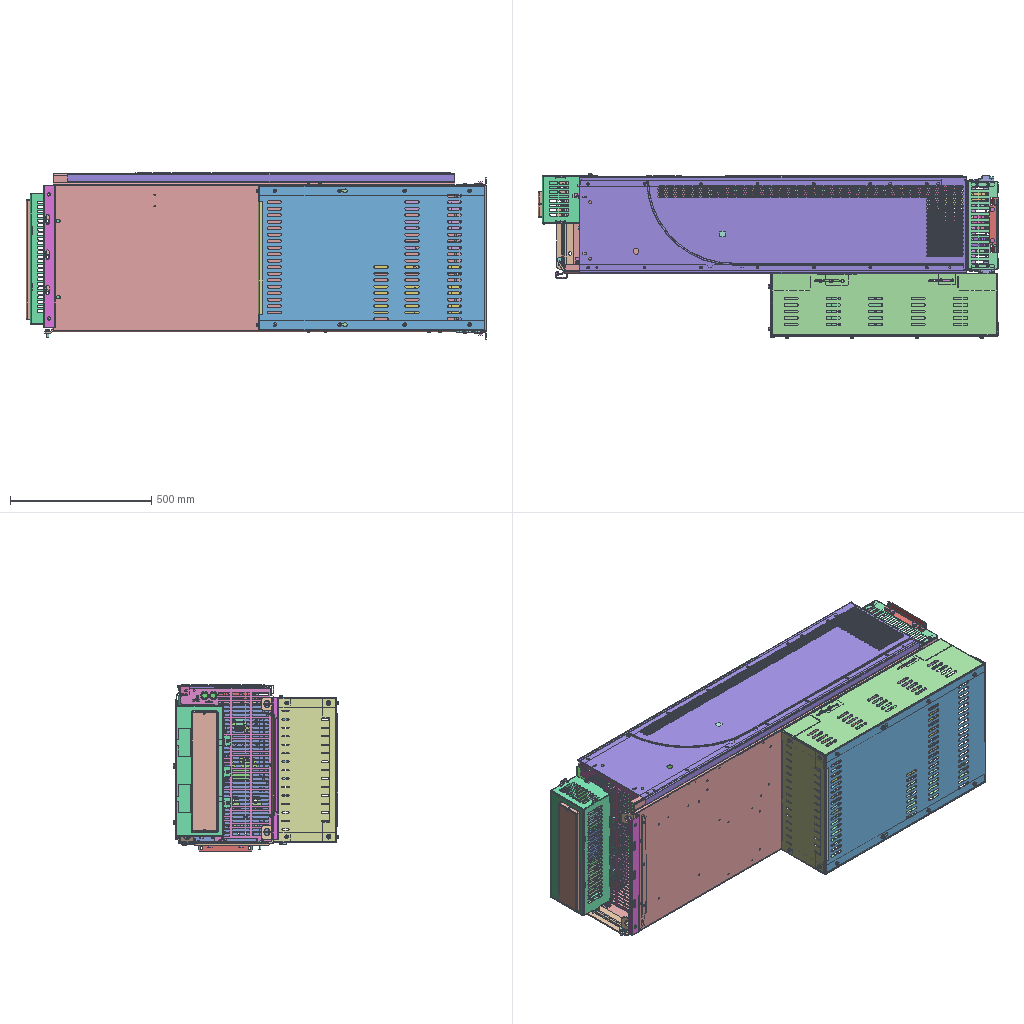Assembly | STEP file | 121 different items | 508 placed | box 1629 x 585 x 589 mm
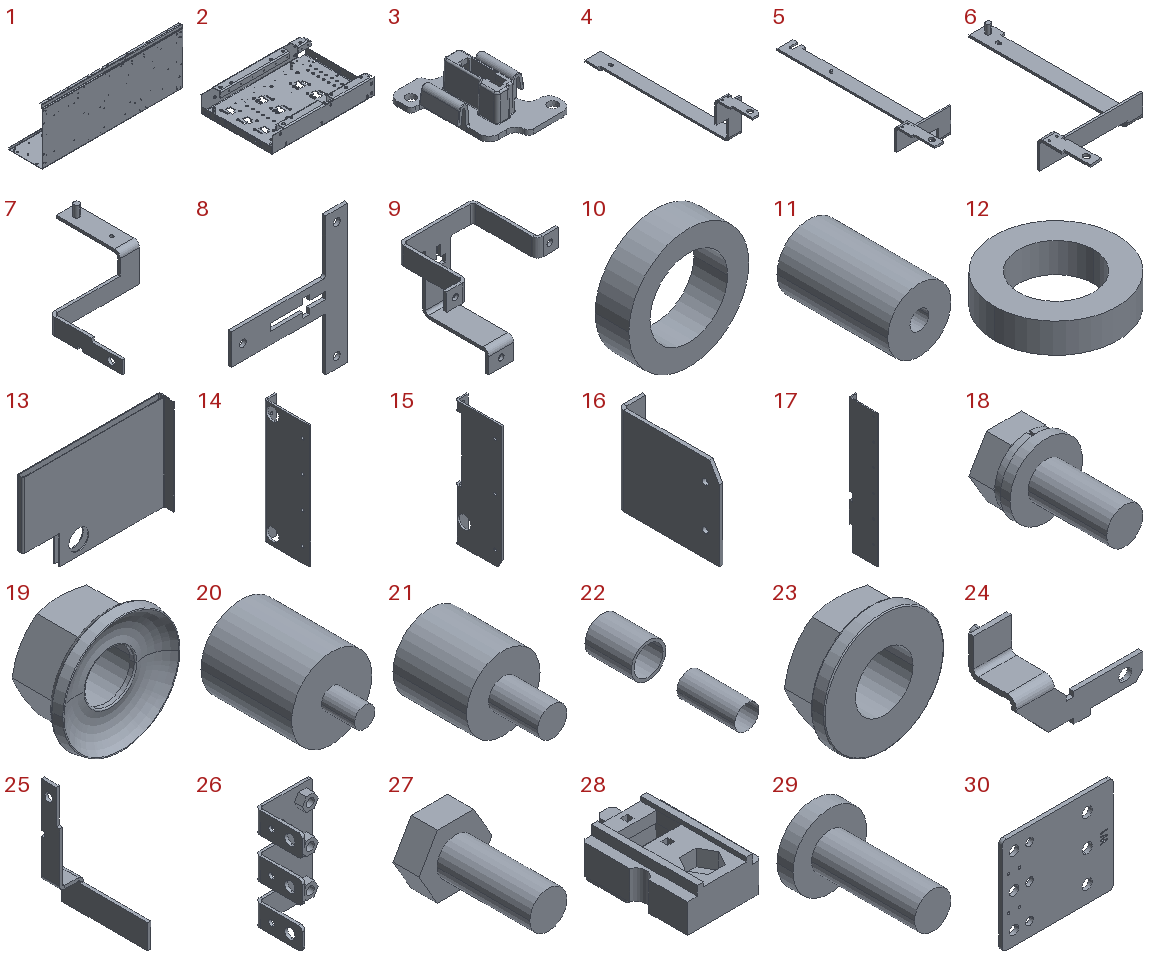Parts list (item | name | quantity | parent item | size | volume):
1 | 64741527 | x1 | - | 1421 x 347.5 x 560 mm | 3305754 mm3
2 | 64560280 | x1 | in 64640828_ASM | 493.5 x 340.5 x 93 mm | 732862 mm3
3 | 64534459 | x6 | in 64640828_ASM | 53 x 64.6 x 22 mm | 11629 mm3
4 | 64562487 | x1 | in 64640828_ASM | 67.1 x 477 x 136.5 mm | 104074 mm3
5 | 64562495 | x1 | in 64640828_ASM | 155.9 x 532.25 x 101.5 mm | 122513 mm3
6 | 64562509 | x1 | in 64640828_ASM | 233.8 x 450 x 76.5 mm | 121760 mm3
7 | 64560433 | x1 | in 64640828_ASM | 159.4 x 245 x 87.7 mm | 67125 mm3
8 | 64562894 | x1 | in 64564421_ASM | 132 x 4 x 157 mm | 27692 mm3
9 | 64562878 | x1 | in 64564421_ASM | 157 x 94 x 132 mm | 57021 mm3
10 | W468 | x1 | in 64564421_ASM | 108.1 x 30.3 x 108.1 mm | 161481 mm3
11 | LIB_58914274 | x3 | in 64564421_ASM | 20 x 35 x 20 mm | 10543 mm3
12 | FERRIITI_104 | x1 | in 64564421_ASM | 104 x 104 x 25 mm | 134441 mm3
13 | 64563181 | x1 | in 64640828_ASM | 151.5 x 16.5 x 101 mm | 21611 mm3
14 | 64605500 | x1 | in 64640828_ASM | 17.5 x 72.5 x 196.5 mm | 40557 mm3
15 | 64605526 | x1 | in 64640828_ASM | 17.5 x 72.5 x 194 mm | 34813 mm3
16 | 64605534 | x1 | in 64640828_ASM | 17.5 x 72.5 x 62.5 mm | 13245 mm3
17 | 64605551 | x1 | in 64640828_ASM | 17.5 x 72.5 x 328 mm | 65751 mm3
18 | LIB_36623110_M6X16 | x25 | in 64640828_ASM, 64667050_68233356_ASM, 68352100_LEFT_ASM, 68374154_ASM | 12 x 20 x 12 mm | 992.686 mm3
19 | KOPRESS_M10 | x5 | in 64640828_ASM | 20.951 x 11.146 x 20.951 mm | 1322 mm3
20 | LIB_57422564 | x1 | in 64640828_ASM | 19.5 x 30 x 19.5 mm | 6600 mm3
21 | SOLID | x2 | in LIB_64610121 | 15 x 25 x 15 mm | 2709 mm3
22 | COMPOUND | x2 | in LIB_64610121 | - | -
23 | LIB_68452317_M6_SERPRESS | x17 | in 64640828_ASM, 64634879_MITTAKUVA_ASM, 64564510_ASM, 64728113_MITTAKUVA_64801082_ASM | 12.5 x 5.2 x 12.5 mm | 351.327 mm3
24 | 64646443 | x1 | in 64640828_ASM | 133.75 x 65.3 x 88.252 mm | 33570 mm3
25 | 64646460 | x1 | in 64640828_ASM | 53.3 x 140.3 x 190 mm | 53459 mm3
26 | 64633074 | x3 | in 64639862_MITTAKUVA_64801082_AF2_ASM, 64639862_MITTAKUVA_64801082_AF1_ASM, 64639862_MITTAKUVA_64801082_AF0_ASM | 60.788 x 52 x 111.5 mm | 28803 mm3
27 | LIB_27897312_M10X25 | x9 | in 64639862_MITTAKUVA_64801082_AF2_ASM, 64639862_MITTAKUVA_64801082_AF1_ASM, 64639862_MITTAKUVA_64801082_AF0_ASM | 19.63 x 32 x 17 mm | 3715 mm3
28 | 58413461 | x9 | in 64639862_MITTAKUVA_64801082_AF2_ASM, 64639862_MITTAKUVA_64801082_AF1_ASM, 64639862_MITTAKUVA_64801082_AF0_ASM | 44 x 71 x 25 mm | 30731 mm3
29 | 4_8X13Y | x36 | in 64639862_MITTAKUVA_64801082_AF2_ASM, 64639862_MITTAKUVA_64801082_AF1_ASM, 64639862_MITTAKUVA_64801082_AF0_ASM | 9.3 x 16.348 x 9.3 mm | 389.106 mm3
30 | SOLID | x1 | in 64634861_AF2 | 144 x 5 x 125 mm | 84805 mm3
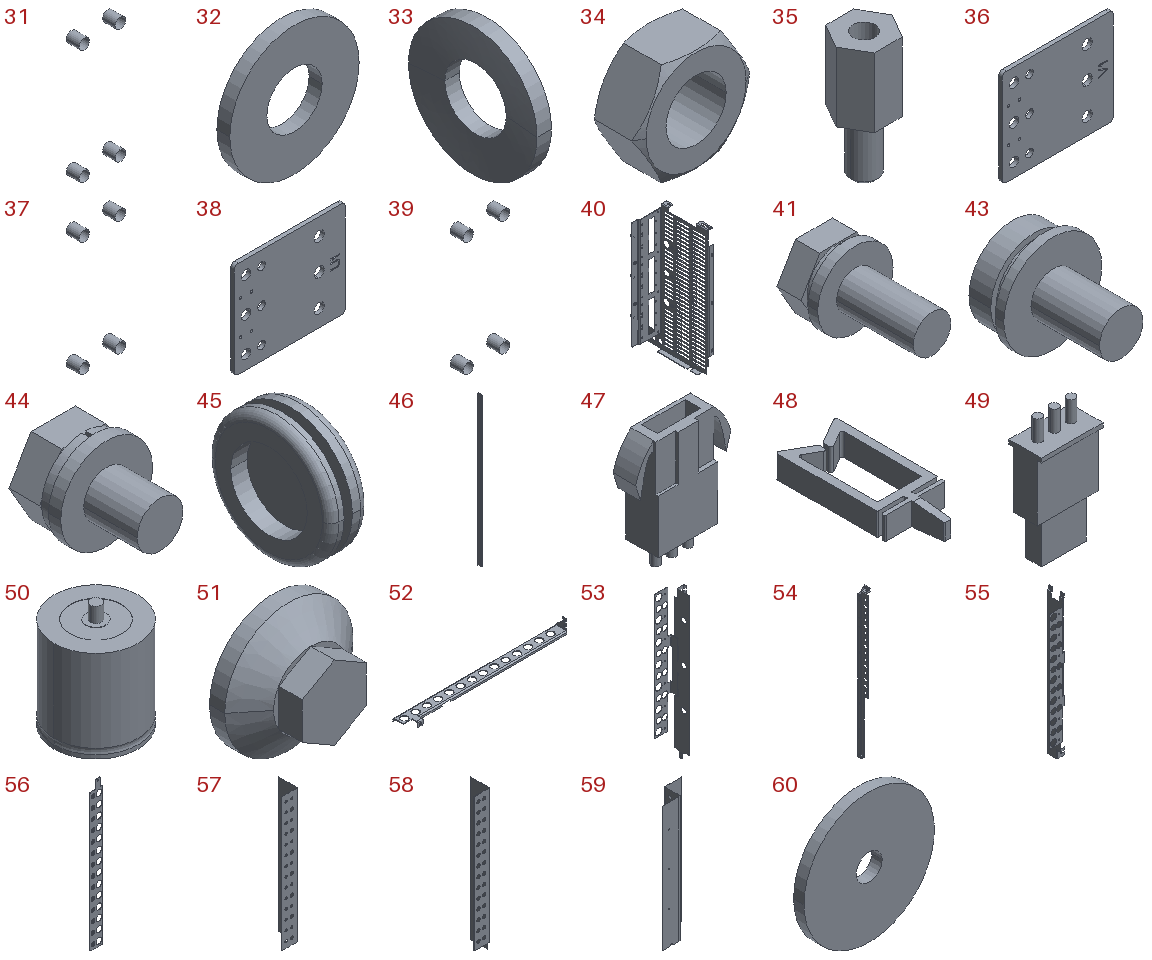31 | COMPOUND | x1 | in 64634861_AF2 | - | -
32 | M10_AALTOLAATTA_DIN125 | x9 | in 64639862_MITTAKUVA_64801082_AF2_ASM, 64639862_MITTAKUVA_64801082_AF1_ASM, 64639862_MITTAKUVA_64801082_AF0_ASM | 25 x 2.5 x 25 mm | 1002 mm3
33 | M10_PAINE_LAATTA | x9 | in 64639862_MITTAKUVA_64801082_AF2_ASM, 64639862_MITTAKUVA_64801082_AF1_ASM, 64639862_MITTAKUVA_64801082_AF0_ASM | 3.1 x 23 x 23 mm | 834.027 mm3
34 | LIB_27044239_HEX_NUT_M10_SIMPLE | x9 | in 64639862_MITTAKUVA_64801082_AF2_ASM, 64639862_MITTAKUVA_64801082_AF1_ASM, 64639862_MITTAKUVA_64801082_AF0_ASM | 19.63 x 8 x 17 mm | 1357 mm3
35 | 58411934 | x3 | in 64639862_MITTAKUVA_64801082_AF2_ASM, 64639862_MITTAKUVA_64801082_AF1_ASM, 64639862_MITTAKUVA_64801082_AF0_ASM | 8.091 x 7 x 18 mm | 467.745 mm3
36 | SOLID | x1 | in 64634861_AF1 | 144 x 5 x 125 mm | 84810 mm3
37 | COMPOUND | x1 | in 64634861_AF1 | - | -
38 | SOLID | x1 | in 64634861_AF0 | 144 x 5 x 125 mm | 84805 mm3
39 | COMPOUND | x1 | in 64634861_AF0 | - | -
40 | 64633091_AF0 | x1 | in 64634879_MITTAKUVA_ASM | 142 x 328 x 554.508 mm | 249746 mm3
41 | LIB_68310857_M10X25 | x25 | in 64634879_MITTAKUVA_ASM, 64667050_68233356_ASM, 64743368_MITTAKUVA_ASM | 20 x 31.4 x 20 mm | 4451 mm3
42 | 64637932_AF0 | x1 | in 64634879_MITTAKUVA_ASM | - | -
43 | LIB_68343097_M4X8 | x13 | in 64634879_MITTAKUVA_ASM | 9 x 11.088 x 9 mm | 282.702 mm3
44 | LIB_36623098_M6X10 | x24 | in 64634879_MITTAKUVA_ASM, 64564528_ASM, 64564536_ASM | 12 x 14 x 12 mm | 823.04 mm3
45 | 60008141 | x2 | in 64634879_MITTAKUVA_ASM | 9.25 x 30 x 30 mm | 3450 mm3
46 | 64685163 | x1 | in 64634879_MITTAKUVA_ASM | 4.361 x 13.946 x 520 mm | 14891 mm3
47 | ELR_03V | x1 | in 64634879_MITTAKUVA_ASM | 23.6 x 8.1 x 29.6 mm | 2454 mm3
48 | 10007151 | x4 | in 64634879_MITTAKUVA_ASM | 15 x 35.134 x 5.6 mm | 963.979 mm3
49 | ELP_03V | x1 | in 64634879_MITTAKUVA_ASM | 14.8 x 10.4 x 29.6 mm | 1903 mm3
50 | 90X105 | x14 | in 64564528_ASM, 64564536_ASM | 90 x 90 x 119.4 mm | 624644 mm3
51 | LIB_58129429 | x14 | in 64564528_ASM, 64564536_ASM | 38 x 19.45 x 38 mm | 10239 mm3
52 | 64560352 | x1 | in 64564528_ASM | 754 x 73 x 68.5 mm | 109655 mm3
53 | 64524275 | x1 | in 64564528_ASM | 128.478 x 101 x 779 mm | 142481 mm3
54 | 64560387 | x1 | in 64564536_ASM | 64 x 67 x 1316 mm | 321357 mm3
55 | 64524283 | x1 | in 64564536_ASM | 126.2 x 96.5 x 835.25 mm | 152034 mm3
56 | 64524267 | x1 | in 64564536_ASM | 64.7 x 6 x 771 mm | 38271 mm3
57 | 64524313 | x1 | in 64564536_ASM | 89 x 104.75 x 746 mm | 102676 mm3
58 | 68379539 | x1 | in 64564536_ASM | 86.7 x 104.75 x 786 mm | 103690 mm3
59 | 64524330 | x1 | in 64564510_ASM | 213.75 x 96 x 768 mm | 116112 mm3
60 | BAR_INSUL_25 | x3 | in 64564510_ASM | 25 x 2 x 25 mm | 942.478 mm3
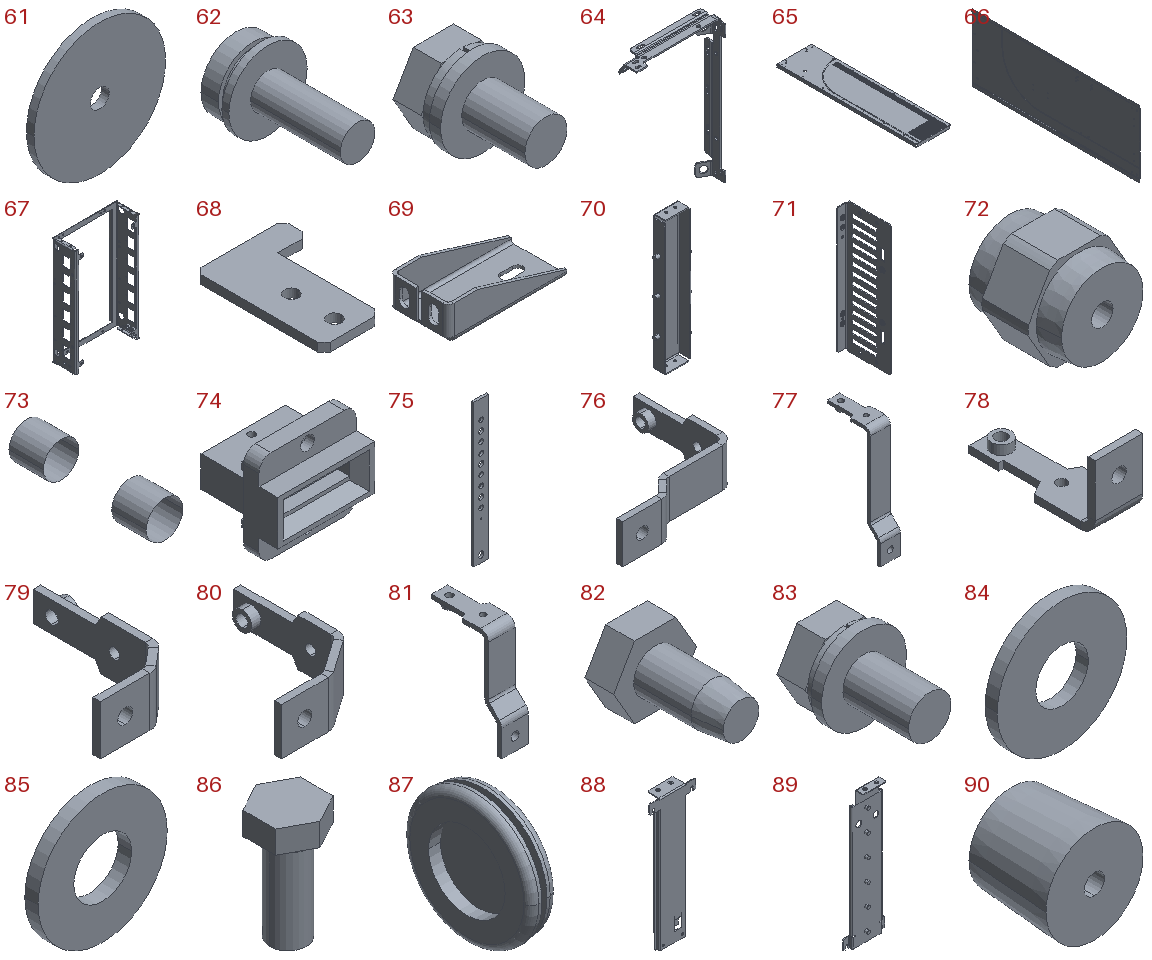61 | BAR_INSUL_35 | x3 | in 64564510_ASM | 35 x 2 x 35 mm | 1885 mm3
62 | LIB_68343071_M4X12 | x3 | in 64564510_ASM | 9 x 15.088 x 9 mm | 332.967 mm3
63 | LIB_36623101_M6X12 | x9 | in 64564510_ASM, 64667050_68233356_ASM, 68341477_ASM | 12 x 16 x 12 mm | 879.589 mm3
64 | 68352819 | x1 | - | 333 x 78.764 x 522.5 mm | 245441 mm3
65 | 64635212 | x1 | - | 342.5 x 1370 x 32 mm | 739959 mm3
66 | 64741551 | x1 | - | 17.8 x 1370 x 552 mm | 1150398 mm3
67 | 64604911 | x1 | in 64667050_68233356_ASM | 312 x 121 x 517 mm | 386207 mm3
68 | 64586793 | x2 | in 64667050_68233356_ASM | 40.84 x 60 x 4 mm | 6725 mm3
69 | 64644335 | x2 | in 64667050_68233356_ASM | 80.5 x 40 x 23.5 mm | 11043 mm3
70 | 64605046 | x1 | in 64667050_68233356_ASM | 80.6 x 27.5 x 306 mm | 73522 mm3
71 | 64586742 | x2 | in 64667050_68233356_ASM | 24 x 108 x 312 mm | 61627 mm3
72 | SOLID | x6 | in LIB_64575945 | 33 x 30 x 30 mm | 19613 mm3
73 | COMPOUND | x6 | in LIB_64575945 | - | -
74 | BUSHING_INSULATOR_CXBY | x12 | in 64667050_68233356_ASM | 56.5 x 48.5 x 53.5 mm | 51454 mm3
75 | 64586807 | x6 | in 64667050_68233356_ASM | 40 x 6 x 397.5 mm | 86530 mm3
76 | 64661426 | x1 | in 64667050_68233356_ASM | 130.6 x 113.5 x 40 mm | 49498 mm3
77 | 64586874 | x1 | in 64667050_68233356_ASM | 40 x 113.5 x 229 mm | 72622 mm3
78 | 64586840 | x1 | in 64667050_68233356_ASM | 40 x 113.5 x 55.6 mm | 32574 mm3
79 | 64586823 | x1 | in 64667050_68233356_ASM | 73.3 x 113.5 x 40 mm | 34639 mm3
80 | 64586815 | x1 | in 64667050_68233356_ASM | 79 x 113.5 x 40 mm | 36513 mm3
81 | 64586785 | x1 | in 64667050_68233356_ASM | 40 x 113.5 x 154 mm | 54622 mm3
82 | TAP_SCREW_DIN7500D_M6X12_TORX | x18 | in 64667050_68233356_ASM | 11.547 x 16 x 10 mm | 601.829 mm3
83 | LIB_36623152_M8X16 | x6 | in 64667050_68233356_ASM | 16 x 21.3 x 16 mm | 2046 mm3
84 | LIB_26379326_WASHER_M12 | x18 | in 64667050_68233356_ASM, 64743368_MITTAKUVA_ASM | 32 x 3 x 32 mm | 2015 mm3
85 | LIB_29542724_CUP_SPRING_M12 | x12 | in 64667050_68233356_ASM, 64743368_MITTAKUVA_ASM | 29 x 3 x 29 mm | 1583 mm3
86 | M12-30 | x6 | in 64667050_68233356_ASM | 19 x 21.1 x 38.1 mm | 5809 mm3
87 | 60008159 | x4 | in 64667050_68233356_ASM | 7.4 x 34.5 x 34.5 mm | 3903 mm3
88 | 64728407 | x1 | in 64728113_MITTAKUVA_64801082_ASM | 144 x 40 x 412 mm | 121719 mm3
89 | 64728377 | x1 | in 64728113_MITTAKUVA_64801082_ASM | 144 x 40.05 x 477.1 mm | 161672 mm3
90 | SOLID | x6 | in 09707255 | 41 x 35 x 41 mm | 39118 mm3
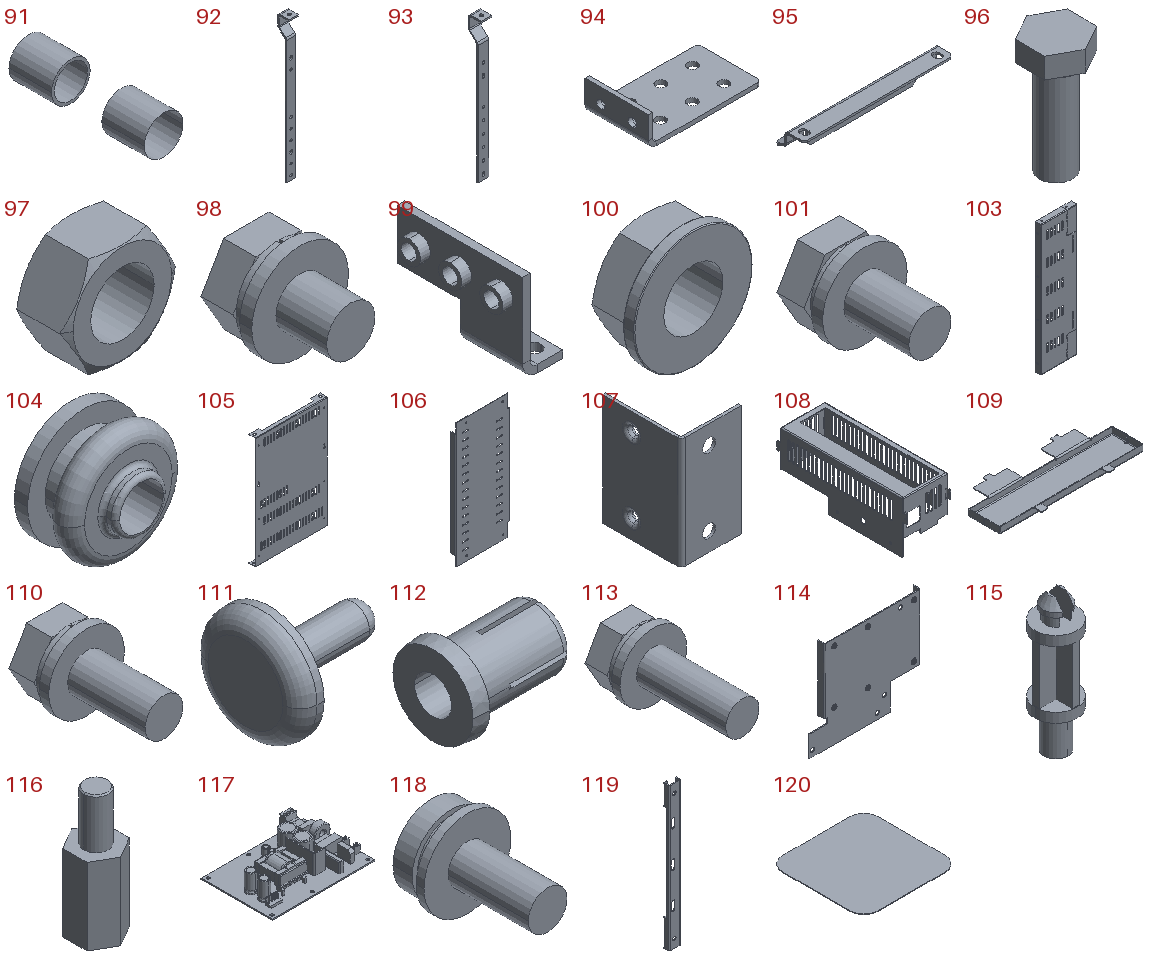91 | COMPOUND | x6 | in 09707255 | - | -
92 | 64805991 | x3 | in 64728113_MITTAKUVA_64801082_ASM | 40 x 51 x 631 mm | 163842 mm3
93 | 64806017 | x3 | in 64728113_MITTAKUVA_64801082_ASM | 40 x 51 x 542 mm | 142711 mm3
94 | 64728105 | x6 | in 64728113_MITTAKUVA_64801082_ASM | 160 x 90 x 44 mm | 97871 mm3
95 | 64668005 | x2 | in 64743368_MITTAKUVA_ASM | 193 x 38.839 x 30 mm | 23240 mm3
96 | M12-35 | x6 | in 64743368_MITTAKUVA_ASM | 19 x 21.1 x 43.1 mm | 6374 mm3
97 | LIB_27044255_HEX_NUT_M12_SIMPLE | x6 | in 64743368_MITTAKUVA_ASM | 21.939 x 10 x 19 mm | 1972 mm3
98 | LIB_36623144_M8X12 | x4 | in 64743368_MITTAKUVA_ASM | 16 x 17.3 x 16 mm | 1844 mm3
99 | 64665871 | x1 | in 64743368_MITTAKUVA_ASM | 39.9 x 100 x 72 mm | 40755 mm3
100 | LIB_68452121_M8_SERPRESS | x2 | in 64743368_MITTAKUVA_ASM | 16 x 6.9 x 16 mm | 740.456 mm3
101 | LIB_68343151_M10X20 | x4 | in 64743368_MITTAKUVA_ASM | 20 x 26.4 x 20 mm | 4058 mm3
102 | 64801082_BRAKE_BUSBAR_ASM | x1 | - | - | -
103 | 68352126 | x2 | in 68352126_ASM | 220 x 35 x 800 mm | 401401 mm3
104 | 233_07_060_230 | x16 | in 68352126_ASM | 13 x 8 x 13 mm | 572.53 mm3
105 | 68352118 | x1 | in 68352100_LEFT_ASM | 514 x 50 x 805 mm | 820655 mm3
106 | 68336503 | x1 | in 68352100_LEFT_ASM | 222.5 x 22 x 512 mm | 244893 mm3
107 | 68332991 | x2 | in 68352100_LEFT_ASM | 32.3 x 42.3 x 60 mm | 6427 mm3
108 | 68341469 | x1 | in 68341477_ASM | 195 x 489 x 195 mm | 358150 mm3
109 | 68341485 | x1 | in 68341477_ASM | 425 x 174 x 22 mm | 133591 mm3
110 | LIB_36623161_M8X20 | x2 | in 68341477_ASM | 16 x 25.3 x 16 mm | 2247 mm3
111 | SR_4060B_1 | x4 | in SRVO_4060_CLOSE_ASM | 8.9 x 8 x 8 mm | 92.138 mm3
112 | SR_4060B_2 | x4 | in SRVO_4060_CLOSE_ASM | 7 x 5.4 x 5.4 mm | 66.144 mm3
113 | LIB_36623179_M8X25 | x1 | - | 16 x 30.3 x 16 mm | 2498 mm3
114 | 68374120 | x1 | in 68374154_ASM | 189.45 x 13.5 x 155 mm | 38724 mm3
115 | MSCBSM_M4_8_01 | x5 | in 68374154_ASM | 7 x 7 x 22.9 mm | 355.891 mm3
116 | 49711204_74 | x1 | in 68374154_ASM | 7 x 8.09 x 20.9 mm | 569.977 mm3
117 | LIB_64668064 | x1 | in 68374154_ASM | 145 x 108.65 x 36.554 mm | 90051 mm3
118 | LIB_28112301_M4X10 | x1 | in 68374154_ASM | 9 x 13.088 x 9 mm | 307.834 mm3
119 | 68377927 | x1 | - | 41 x 21.5 x 500 mm | 101475 mm3
120 | 68423252 | x1 | - | 20 x 20 x 0.125 mm | 49.034 mm3
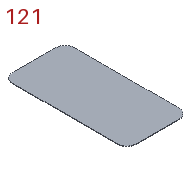121 | 68437831 | x1 | - | 20 x 40 x 0.125 mm | 99.034 mm3
Placements (level | parent | child | x y z in mm | rotation matrix by rows), first 274 of 546 lines:
1 | subassembly 2 | 64741527 | 0.0 0.0 0.0 | 1 0 0 0 1 0 0 0 1
1 | subassembly 2 | 64640828_ASM | 683.0 176.0 0.5 | 0 -1 0 1 0 0 0 0 1
2 | 64640828_ASM | 64560280 | -6.0 0.0 -1.0 | 0 1 0 0 0 -1 -1 0 0
2 | 64640828_ASM | 64534459 | 106.93 5.5 126.6 | 0 1 0 0 0 -1 -1 0 0
2 | 64640828_ASM | 64534459 | 26.23 5.5 126.6 | 0 1 0 0 0 -1 -1 0 0
2 | 64640828_ASM | 64534459 | -52.77 5.5 126.6 | 0 1 0 0 0 -1 -1 0 0
2 | 64640828_ASM | 64562487 | 91.18 29.5 -42.5 | 1 0 0 0 1 0 0 0 1
2 | 64640828_ASM | 64562495 | 50.78 35.5 -42.5 | 1 0 0 0 1 0 0 0 1
2 | 64640828_ASM | 64562509 | 11.83 41.5 -43.25 | 1 0 0 0 1 0 0 0 1
2 | 64640828_ASM | 64560433 | 39.33 60.5 -32.8 | 0 0 1 0 1 0 -1 0 0
2 | 64640828_ASM | 64564421_ASM | 108.8 41.5 -94.0 | 1 0 0 0 1 0 0 0 1
3 | 64564421_ASM | 64562894 | 0.0 0.0 0.0 | 1 0 0 0 1 0 0 0 1
3 | 64564421_ASM | 64562878 | -4.07 94.0 0.0 | 0 0 1 0 1 0 -1 0 0
3 | 64564421_ASM | W468 | -1.07 0.0 0.0 | 1 0 0 0 1 0 0 0 1
3 | 64564421_ASM | LIB_58914274 | 32.43 -39.0 66.0 | 1 0 0 0 1 0 0 0 1
3 | 64564421_ASM | LIB_58914274 | -74.57 -39.0 0.0 | 1 0 0 0 1 0 0 0 1
3 | 64564421_ASM | LIB_58914274 | 32.43 -39.0 -66.0 | 1 0 0 0 1 0 0 0 1
3 | 64564421_ASM | FERRIITI_104 | -1.07 90.0 0.0 | 1 0 0 0 0 -1 0 1 0
2 | 64640828_ASM | 64563181 | 123.83 30.5 -8.0 | 1 0 0 0 1 0 0 0 1
2 | 64640828_ASM | 64605500 | -139.0 -2.5 149.0 | 1 0 0 0 1 0 0 0 1
2 | 64640828_ASM | 64605526 | -139.0 -2.5 -89.5 | 1 0 0 0 1 0 0 0 1
2 | 64640828_ASM | 64605534 | 130.5 -2.5 -283.5 | -1 0 0 0 1 0 0 0 -1
2 | 64640828_ASM | 64605551 | 130.5 -2.5 -179.0 | -1 0 0 0 1 0 0 0 -1
2 | 64640828_ASM | LIB_36623110_M6X16 | 34.23 50.5 -94.0 | 1 0 0 0 1 0 0 0 1
2 | 64640828_ASM | LIB_36623110_M6X16 | 141.23 48.5 -160.0 | 1 0 0 0 1 0 0 0 1
2 | 64640828_ASM | LIB_36623110_M6X16 | 141.23 48.5 -28.0 | 1 0 0 0 1 0 0 0 1
2 | 64640828_ASM | KOPRESS_M10 | 84.93 157.5 -15.3 | 0 1 0 -1 0 0 0 0 1
2 | 64640828_ASM | KOPRESS_M10 | 107.23 392.0 -124.4 | 1 0 0 0 0 1 0 -1 0
2 | 64640828_ASM | KOPRESS_M10 | 114.03 365.0 -63.6 | -1 0 0 0 0 1 0 1 0
2 | 64640828_ASM | LIB_57422564 | 107.0 2.5 -73.5 | 1 0 0 0 1 0 0 0 1
2 | 64640828_ASM | LIB_64610121 | 107.23 335.5 -76.5 | 1 0 0 0 0 1 0 -1 0
3 | LIB_64610121 | SOLID | 0.0 0.0 0.0 | 1 0 0 0 1 0 0 0 1
3 | LIB_64610121 | COMPOUND | 0.0 0.0 0.0 | 1 0 0 0 1 0 0 0 1
2 | 64640828_ASM | LIB_64610121 | 107.23 362.5 -111.5 | -1 0 0 0 0 1 0 1 0
3 | LIB_64610121 | SOLID | 0.0 0.0 0.0 | 1 0 0 0 1 0 0 0 1
3 | LIB_64610121 | COMPOUND | 0.0 0.0 0.0 | 1 0 0 0 1 0 0 0 1
2 | 64640828_ASM | LIB_68452317_M6_SERPRESS | 107.23 335.5 -70.1 | -1 0 0 0 0 1 0 1 0
2 | 64640828_ASM | LIB_68452317_M6_SERPRESS | 107.23 362.5 -117.9 | 1 0 0 0 0 1 0 -1 0
2 | 64640828_ASM | 64534459 | -87.9 5.5 -5.0 | 0 -1 0 0 0 -1 1 0 0
2 | 64640828_ASM | 64534459 | -10.0 5.5 -5.0 | 0 -1 0 0 0 -1 1 0 0
2 | 64640828_ASM | 64534459 | 70.8 5.5 -5.0 | 0 -1 0 0 0 -1 1 0 0
2 | 64640828_ASM | 64646443 | 33.0 66.25 126.5 | 0 0 -1 -1 0 0 0 1 0
2 | 64640828_ASM | 64646460 | -70.0 -67.5 126.5 | 0 -1 0 0 0 -1 1 0 0
2 | 64640828_ASM | KOPRESS_M10 | 49.5 102.5 166.7 | -1 0 0 0 0 1 0 1 0
2 | 64640828_ASM | KOPRESS_M10 | 46.748 46.25 178.7 | -1 0 0 0 0 1 0 1 0
1 | subassembly 2 | 64634879_MITTAKUVA_ASM | -563.5 197.095 116.25 | 0 -1 0 -1 0 0 0 0 -1
2 | 64634879_MITTAKUVA_ASM | 64639862_MITTAKUVA_64801082_AF2_ASM | 0.0 0.0 0.0 | 1 0 0 0 1 0 0 0 1
3 | 64639862_MITTAKUVA_64801082_AF2_ASM | 64633074 | 0.0 0.0 0.0 | 1 0 0 0 1 0 0 0 1
3 | 64639862_MITTAKUVA_64801082_AF2_ASM | LIB_27897312_M10X25 | -37.065 -35.7 -44.5 | 0 1 0 1 0 0 0 0 -1
3 | 64639862_MITTAKUVA_64801082_AF2_ASM | LIB_27897312_M10X25 | -37.065 -35.7 0.0 | 0 1 0 1 0 0 0 0 -1
3 | 64639862_MITTAKUVA_64801082_AF2_ASM | LIB_27897312_M10X25 | -37.065 -35.7 44.5 | 0 1 0 1 0 0 0 0 -1
3 | 64639862_MITTAKUVA_64801082_AF2_ASM | 58413461 | -28.315 -18.0 -44.5 | 0 0 -1 0 1 0 1 0 0
3 | 64639862_MITTAKUVA_64801082_AF2_ASM | 58413461 | -28.315 -18.0 0.0 | 0 0 -1 0 1 0 1 0 0
3 | 64639862_MITTAKUVA_64801082_AF2_ASM | 58413461 | -28.315 -18.0 44.5 | 0 0 -1 0 1 0 1 0 0
3 | 64639862_MITTAKUVA_64801082_AF2_ASM | 4_8X13Y | -11.565 -42.0 -27.5 | 0 1 0 -1 0 0 0 0 1
3 | 64639862_MITTAKUVA_64801082_AF2_ASM | 4_8X13Y | -11.565 -42.0 17.0 | 0 1 0 -1 0 0 0 0 1
3 | 64639862_MITTAKUVA_64801082_AF2_ASM | 4_8X13Y | -11.565 -42.0 61.5 | 0 1 0 -1 0 0 0 0 1
3 | 64639862_MITTAKUVA_64801082_AF2_ASM | 4_8X13Y | -11.565 -42.0 -61.5 | 0 1 0 -1 0 0 0 0 1
3 | 64639862_MITTAKUVA_64801082_AF2_ASM | 4_8X13Y | -11.565 -42.0 -17.0 | 0 1 0 -1 0 0 0 0 1
3 | 64639862_MITTAKUVA_64801082_AF2_ASM | 4_8X13Y | -11.565 -42.0 27.5 | 0 1 0 -1 0 0 0 0 1
3 | 64639862_MITTAKUVA_64801082_AF2_ASM | 4_8X13Y | -11.565 17.5 -44.5 | 0 1 0 -1 0 0 0 0 1
3 | 64639862_MITTAKUVA_64801082_AF2_ASM | 4_8X13Y | -11.565 17.5 0.0 | 0 1 0 -1 0 0 0 0 1
3 | 64639862_MITTAKUVA_64801082_AF2_ASM | 4_8X13Y | -11.565 17.5 44.5 | 0 1 0 -1 0 0 0 0 1
3 | 64639862_MITTAKUVA_64801082_AF2_ASM | 4_8X13Y | -43.565 -15.5 -44.5 | 0 -1 0 1 0 0 0 0 1
3 | 64639862_MITTAKUVA_64801082_AF2_ASM | 4_8X13Y | -43.565 -15.5 0.0 | 0 -1 0 1 0 0 0 0 1
3 | 64639862_MITTAKUVA_64801082_AF2_ASM | 4_8X13Y | -43.565 -15.5 44.5 | 0 -1 0 1 0 0 0 0 1
3 | 64639862_MITTAKUVA_64801082_AF2_ASM | 64634861_AF2 | -45.065 21.3 0.0 | 0 1 0 1 0 0 0 0 -1
4 | 64634861_AF2 | SOLID | 0.0 0.0 0.0 | 1 0 0 0 1 0 0 0 1
4 | 64634861_AF2 | COMPOUND | 0.0 0.0 0.0 | 1 0 0 0 1 0 0 0 1
3 | 64639862_MITTAKUVA_64801082_AF2_ASM | M10_AALTOLAATTA_DIN125 | -47.565 -35.7 -44.5 | 0 1 0 -1 0 0 0 0 1
3 | 64639862_MITTAKUVA_64801082_AF2_ASM | M10_AALTOLAATTA_DIN125 | -47.565 -35.7 0.0 | 0 1 0 -1 0 0 0 0 1
3 | 64639862_MITTAKUVA_64801082_AF2_ASM | M10_AALTOLAATTA_DIN125 | -47.565 -35.7 44.5 | 0 1 0 -1 0 0 0 0 1
3 | 64639862_MITTAKUVA_64801082_AF2_ASM | M10_PAINE_LAATTA | -47.065 -35.7 -44.5 | -1 0 0 0 -1 0 0 0 1
3 | 64639862_MITTAKUVA_64801082_AF2_ASM | M10_PAINE_LAATTA | -47.065 -35.7 0.0 | -1 0 0 0 -1 0 0 0 1
3 | 64639862_MITTAKUVA_64801082_AF2_ASM | M10_PAINE_LAATTA | -47.065 -35.7 44.5 | -1 0 0 0 -1 0 0 0 1
3 | 64639862_MITTAKUVA_64801082_AF2_ASM | LIB_27044239_HEX_NUT_M10_SIMPLE | -58.065 -35.7 -44.5 | 0 1 0 -1 0 0 0 0 1
3 | 64639862_MITTAKUVA_64801082_AF2_ASM | LIB_27044239_HEX_NUT_M10_SIMPLE | -58.065 -35.7 0.0 | 0 1 0 -1 0 0 0 0 1
3 | 64639862_MITTAKUVA_64801082_AF2_ASM | LIB_27044239_HEX_NUT_M10_SIMPLE | -58.065 -35.7 44.5 | 0 1 0 -1 0 0 0 0 1
3 | 64639862_MITTAKUVA_64801082_AF2_ASM | 58411934 | -45.065 -28.7 -22.25 | 0 0 -1 -1 0 0 0 1 0
2 | 64634879_MITTAKUVA_ASM | 64639862_MITTAKUVA_64801082_AF1_ASM | 0.0 0.0 151.75 | 1 0 0 0 1 0 0 0 1
3 | 64639862_MITTAKUVA_64801082_AF1_ASM | 64633074 | 0.0 0.0 0.0 | 1 0 0 0 1 0 0 0 1
3 | 64639862_MITTAKUVA_64801082_AF1_ASM | LIB_27897312_M10X25 | -37.065 -35.7 -44.5 | 0 1 0 1 0 0 0 0 -1
3 | 64639862_MITTAKUVA_64801082_AF1_ASM | LIB_27897312_M10X25 | -37.065 -35.7 0.0 | 0 1 0 1 0 0 0 0 -1
3 | 64639862_MITTAKUVA_64801082_AF1_ASM | LIB_27897312_M10X25 | -37.065 -35.7 44.5 | 0 1 0 1 0 0 0 0 -1
3 | 64639862_MITTAKUVA_64801082_AF1_ASM | 58413461 | -28.315 -18.0 -44.5 | 0 0 -1 0 1 0 1 0 0
3 | 64639862_MITTAKUVA_64801082_AF1_ASM | 58413461 | -28.315 -18.0 0.0 | 0 0 -1 0 1 0 1 0 0
3 | 64639862_MITTAKUVA_64801082_AF1_ASM | 58413461 | -28.315 -18.0 44.5 | 0 0 -1 0 1 0 1 0 0
3 | 64639862_MITTAKUVA_64801082_AF1_ASM | 4_8X13Y | -11.565 -42.0 -27.5 | 0 1 0 -1 0 0 0 0 1
3 | 64639862_MITTAKUVA_64801082_AF1_ASM | 4_8X13Y | -11.565 -42.0 17.0 | 0 1 0 -1 0 0 0 0 1
3 | 64639862_MITTAKUVA_64801082_AF1_ASM | 4_8X13Y | -11.565 -42.0 61.5 | 0 1 0 -1 0 0 0 0 1
3 | 64639862_MITTAKUVA_64801082_AF1_ASM | 4_8X13Y | -11.565 -42.0 -61.5 | 0 1 0 -1 0 0 0 0 1
3 | 64639862_MITTAKUVA_64801082_AF1_ASM | 4_8X13Y | -11.565 -42.0 -17.0 | 0 1 0 -1 0 0 0 0 1
3 | 64639862_MITTAKUVA_64801082_AF1_ASM | 4_8X13Y | -11.565 -42.0 27.5 | 0 1 0 -1 0 0 0 0 1
3 | 64639862_MITTAKUVA_64801082_AF1_ASM | 4_8X13Y | -11.565 17.5 -44.5 | 0 1 0 -1 0 0 0 0 1
3 | 64639862_MITTAKUVA_64801082_AF1_ASM | 4_8X13Y | -11.565 17.5 0.0 | 0 1 0 -1 0 0 0 0 1
3 | 64639862_MITTAKUVA_64801082_AF1_ASM | 4_8X13Y | -11.565 17.5 44.5 | 0 1 0 -1 0 0 0 0 1
3 | 64639862_MITTAKUVA_64801082_AF1_ASM | 4_8X13Y | -43.565 -15.5 -44.5 | 0 -1 0 1 0 0 0 0 1
3 | 64639862_MITTAKUVA_64801082_AF1_ASM | 4_8X13Y | -43.565 -15.5 0.0 | 0 -1 0 1 0 0 0 0 1
3 | 64639862_MITTAKUVA_64801082_AF1_ASM | 4_8X13Y | -43.565 -15.5 44.5 | 0 -1 0 1 0 0 0 0 1
3 | 64639862_MITTAKUVA_64801082_AF1_ASM | 64634861_AF1 | -45.065 21.3 0.0 | 0 1 0 1 0 0 0 0 -1
4 | 64634861_AF1 | SOLID | 0.0 0.0 0.0 | 1 0 0 0 1 0 0 0 1
4 | 64634861_AF1 | COMPOUND | 0.0 0.0 0.0 | 1 0 0 0 1 0 0 0 1
3 | 64639862_MITTAKUVA_64801082_AF1_ASM | M10_AALTOLAATTA_DIN125 | -47.565 -35.7 -44.5 | 0 1 0 -1 0 0 0 0 1
3 | 64639862_MITTAKUVA_64801082_AF1_ASM | M10_AALTOLAATTA_DIN125 | -47.565 -35.7 0.0 | 0 1 0 -1 0 0 0 0 1
3 | 64639862_MITTAKUVA_64801082_AF1_ASM | M10_AALTOLAATTA_DIN125 | -47.565 -35.7 44.5 | 0 1 0 -1 0 0 0 0 1
3 | 64639862_MITTAKUVA_64801082_AF1_ASM | M10_PAINE_LAATTA | -47.065 -35.7 -44.5 | -1 0 0 0 -1 0 0 0 1
3 | 64639862_MITTAKUVA_64801082_AF1_ASM | M10_PAINE_LAATTA | -47.065 -35.7 0.0 | -1 0 0 0 -1 0 0 0 1
3 | 64639862_MITTAKUVA_64801082_AF1_ASM | M10_PAINE_LAATTA | -47.065 -35.7 44.5 | -1 0 0 0 -1 0 0 0 1
3 | 64639862_MITTAKUVA_64801082_AF1_ASM | LIB_27044239_HEX_NUT_M10_SIMPLE | -58.065 -35.7 -44.5 | 0 1 0 -1 0 0 0 0 1
3 | 64639862_MITTAKUVA_64801082_AF1_ASM | LIB_27044239_HEX_NUT_M10_SIMPLE | -58.065 -35.7 0.0 | 0 1 0 -1 0 0 0 0 1
3 | 64639862_MITTAKUVA_64801082_AF1_ASM | LIB_27044239_HEX_NUT_M10_SIMPLE | -58.065 -35.7 44.5 | 0 1 0 -1 0 0 0 0 1
3 | 64639862_MITTAKUVA_64801082_AF1_ASM | 58411934 | -45.065 -28.7 -22.25 | 0 0 -1 -1 0 0 0 1 0
2 | 64634879_MITTAKUVA_ASM | 64639862_MITTAKUVA_64801082_AF0_ASM | 0.0 0.0 303.5 | 1 0 0 0 1 0 0 0 1
3 | 64639862_MITTAKUVA_64801082_AF0_ASM | 64633074 | 0.0 0.0 0.0 | 1 0 0 0 1 0 0 0 1
3 | 64639862_MITTAKUVA_64801082_AF0_ASM | LIB_27897312_M10X25 | -37.065 -35.7 -44.5 | 0 1 0 1 0 0 0 0 -1
3 | 64639862_MITTAKUVA_64801082_AF0_ASM | LIB_27897312_M10X25 | -37.065 -35.7 0.0 | 0 1 0 1 0 0 0 0 -1
3 | 64639862_MITTAKUVA_64801082_AF0_ASM | LIB_27897312_M10X25 | -37.065 -35.7 44.5 | 0 1 0 1 0 0 0 0 -1
3 | 64639862_MITTAKUVA_64801082_AF0_ASM | 58413461 | -28.315 -18.0 -44.5 | 0 0 -1 0 1 0 1 0 0
3 | 64639862_MITTAKUVA_64801082_AF0_ASM | 58413461 | -28.315 -18.0 0.0 | 0 0 -1 0 1 0 1 0 0
3 | 64639862_MITTAKUVA_64801082_AF0_ASM | 58413461 | -28.315 -18.0 44.5 | 0 0 -1 0 1 0 1 0 0
3 | 64639862_MITTAKUVA_64801082_AF0_ASM | 4_8X13Y | -11.565 -42.0 -27.5 | 0 1 0 -1 0 0 0 0 1
3 | 64639862_MITTAKUVA_64801082_AF0_ASM | 4_8X13Y | -11.565 -42.0 17.0 | 0 1 0 -1 0 0 0 0 1
3 | 64639862_MITTAKUVA_64801082_AF0_ASM | 4_8X13Y | -11.565 -42.0 61.5 | 0 1 0 -1 0 0 0 0 1
3 | 64639862_MITTAKUVA_64801082_AF0_ASM | 4_8X13Y | -11.565 -42.0 -61.5 | 0 1 0 -1 0 0 0 0 1
3 | 64639862_MITTAKUVA_64801082_AF0_ASM | 4_8X13Y | -11.565 -42.0 -17.0 | 0 1 0 -1 0 0 0 0 1
3 | 64639862_MITTAKUVA_64801082_AF0_ASM | 4_8X13Y | -11.565 -42.0 27.5 | 0 1 0 -1 0 0 0 0 1
3 | 64639862_MITTAKUVA_64801082_AF0_ASM | 4_8X13Y | -11.565 17.5 -44.5 | 0 1 0 -1 0 0 0 0 1
3 | 64639862_MITTAKUVA_64801082_AF0_ASM | 4_8X13Y | -11.565 17.5 0.0 | 0 1 0 -1 0 0 0 0 1
3 | 64639862_MITTAKUVA_64801082_AF0_ASM | 4_8X13Y | -11.565 17.5 44.5 | 0 1 0 -1 0 0 0 0 1
3 | 64639862_MITTAKUVA_64801082_AF0_ASM | 4_8X13Y | -43.565 -15.5 -44.5 | 0 -1 0 1 0 0 0 0 1
3 | 64639862_MITTAKUVA_64801082_AF0_ASM | 4_8X13Y | -43.565 -15.5 0.0 | 0 -1 0 1 0 0 0 0 1
3 | 64639862_MITTAKUVA_64801082_AF0_ASM | 4_8X13Y | -43.565 -15.5 44.5 | 0 -1 0 1 0 0 0 0 1
3 | 64639862_MITTAKUVA_64801082_AF0_ASM | 64634861_AF0 | -45.065 21.3 0.0 | 0 1 0 1 0 0 0 0 -1
4 | 64634861_AF0 | SOLID | 0.0 0.0 0.0 | 1 0 0 0 1 0 0 0 1
4 | 64634861_AF0 | COMPOUND | 0.0 0.0 0.0 | 1 0 0 0 1 0 0 0 1
3 | 64639862_MITTAKUVA_64801082_AF0_ASM | M10_AALTOLAATTA_DIN125 | -47.565 -35.7 -44.5 | 0 1 0 -1 0 0 0 0 1
3 | 64639862_MITTAKUVA_64801082_AF0_ASM | M10_AALTOLAATTA_DIN125 | -47.565 -35.7 0.0 | 0 1 0 -1 0 0 0 0 1
3 | 64639862_MITTAKUVA_64801082_AF0_ASM | M10_AALTOLAATTA_DIN125 | -47.565 -35.7 44.5 | 0 1 0 -1 0 0 0 0 1
3 | 64639862_MITTAKUVA_64801082_AF0_ASM | M10_PAINE_LAATTA | -47.065 -35.7 -44.5 | -1 0 0 0 -1 0 0 0 1
3 | 64639862_MITTAKUVA_64801082_AF0_ASM | M10_PAINE_LAATTA | -47.065 -35.7 0.0 | -1 0 0 0 -1 0 0 0 1
3 | 64639862_MITTAKUVA_64801082_AF0_ASM | M10_PAINE_LAATTA | -47.065 -35.7 44.5 | -1 0 0 0 -1 0 0 0 1
3 | 64639862_MITTAKUVA_64801082_AF0_ASM | LIB_27044239_HEX_NUT_M10_SIMPLE | -58.065 -35.7 -44.5 | 0 1 0 -1 0 0 0 0 1
3 | 64639862_MITTAKUVA_64801082_AF0_ASM | LIB_27044239_HEX_NUT_M10_SIMPLE | -58.065 -35.7 0.0 | 0 1 0 -1 0 0 0 0 1
3 | 64639862_MITTAKUVA_64801082_AF0_ASM | LIB_27044239_HEX_NUT_M10_SIMPLE | -58.065 -35.7 44.5 | 0 1 0 -1 0 0 0 0 1
3 | 64639862_MITTAKUVA_64801082_AF0_ASM | 58411934 | -45.065 -28.7 -22.25 | 0 0 -1 -1 0 0 0 1 0
2 | 64634879_MITTAKUVA_ASM | 64633091_AF0 | 194.595 38.8 151.4 | 0 -1 0 1 0 0 0 0 1
2 | 64634879_MITTAKUVA_ASM | LIB_68310857_M10X25 | 9.0 13.6 41.75 | 1 0 0 0 1 0 0 0 1
2 | 64634879_MITTAKUVA_ASM | LIB_68310857_M10X25 | 9.0 13.6 151.75 | 1 0 0 0 1 0 0 0 1
2 | 64634879_MITTAKUVA_ASM | LIB_68310857_M10X25 | 9.0 13.6 261.75 | 1 0 0 0 1 0 0 0 1
2 | 64634879_MITTAKUVA_ASM | LIB_68452317_M6_SERPRESS | 189.195 51.8 126.4 | 0 -1 0 1 0 0 0 0 1
2 | 64634879_MITTAKUVA_ASM | LIB_68452317_M6_SERPRESS | 5.095 51.8 398.858 | 1 0 0 0 0 1 0 -1 0
2 | 64634879_MITTAKUVA_ASM | LIB_68452317_M6_SERPRESS | 154.595 51.8 398.858 | 1 0 0 0 0 1 0 -1 0
2 | 64634879_MITTAKUVA_ASM | LIB_68452317_M6_SERPRESS | 189.195 51.8 306.4 | 0 -1 0 1 0 0 0 0 1
2 | 64634879_MITTAKUVA_ASM | LIB_68452317_M6_SERPRESS | 189.195 51.8 -53.6 | 0 -1 0 1 0 0 0 0 1
2 | 64634879_MITTAKUVA_ASM | 64637932_AF0 | 22.595 43.3 126.258 | -1 0 0 0 1 0 0 0 -1
2 | 64634879_MITTAKUVA_ASM | LIB_68343097_M4X8 | -46.065 -28.7 174.0 | 0 -1 0 1 0 0 0 0 1
2 | 64634879_MITTAKUVA_ASM | LIB_68343097_M4X8 | -46.065 -28.7 325.75 | 0 -1 0 1 0 0 0 0 1
2 | 64634879_MITTAKUVA_ASM | LIB_36623098_M6X10 | -28.455 -68.2 74.55 | 0 -1 0 1 0 0 0 0 1
2 | 64634879_MITTAKUVA_ASM | LIB_36623098_M6X10 | -28.455 -68.2 229.55 | 0 -1 0 1 0 0 0 0 1
2 | 64634879_MITTAKUVA_ASM | LIB_68343097_M4X8 | -36.455 -71.2 24.4 | 0 -1 0 1 0 0 0 0 1
2 | 64634879_MITTAKUVA_ASM | LIB_68343097_M4X8 | -36.455 -71.2 176.4 | 0 -1 0 1 0 0 0 0 1
2 | 64634879_MITTAKUVA_ASM | LIB_68343097_M4X8 | -36.455 -71.2 328.4 | 0 -1 0 1 0 0 0 0 1
2 | 64634879_MITTAKUVA_ASM | LIB_68343097_M4X8 | -4.0 -1.0 -21.75 | -1 0 0 0 -1 0 0 0 1
2 | 64634879_MITTAKUVA_ASM | LIB_68343097_M4X8 | -4.0 -1.0 21.75 | -1 0 0 0 -1 0 0 0 1
2 | 64634879_MITTAKUVA_ASM | LIB_68343097_M4X8 | -4.0 -1.0 130.0 | -1 0 0 0 -1 0 0 0 1
2 | 64634879_MITTAKUVA_ASM | LIB_68343097_M4X8 | -4.0 -1.0 173.5 | -1 0 0 0 -1 0 0 0 1
2 | 64634879_MITTAKUVA_ASM | LIB_68343097_M4X8 | -4.0 -1.0 325.25 | -1 0 0 0 -1 0 0 0 1
2 | 64634879_MITTAKUVA_ASM | LIB_68343097_M4X8 | -4.0 -1.0 281.75 | -1 0 0 0 -1 0 0 0 1
2 | 64634879_MITTAKUVA_ASM | 60008141 | -17.405 39.8 -118.6 | 0 -1 0 1 0 0 0 0 1
2 | 64634879_MITTAKUVA_ASM | 60008141 | -48.405 39.8 -118.6 | 0 1 0 -1 0 0 0 0 1
2 | 64634879_MITTAKUVA_ASM | 64685163 | -64.905 -10.197 126.758 | 0 1 0 -1 0 0 0 0 1
2 | 64634879_MITTAKUVA_ASM | ELR_03V | -78.805 50.1 -105.25 | -1 0 0 0 0 1 0 1 0
2 | 64634879_MITTAKUVA_ASM | 10007151 | -15.055 26.8 373.6 | 0 1 0 -1 0 0 0 0 1
2 | 64634879_MITTAKUVA_ASM | 10007151 | -15.055 26.8 223.6 | 0 1 0 -1 0 0 0 0 1
2 | 64634879_MITTAKUVA_ASM | 10007151 | -15.055 26.8 73.6 | 0 1 0 -1 0 0 0 0 1
2 | 64634879_MITTAKUVA_ASM | 10007151 | -15.055 26.8 -76.4 | 0 1 0 -1 0 0 0 0 1
2 | 64634879_MITTAKUVA_ASM | ELP_03V | -78.805 63.7 -98.15 | 1 0 0 0 0 1 0 -1 0
2 | 64634879_MITTAKUVA_ASM | LIB_68343097_M4X8 | -56.065 -28.7 -22.25 | 0 -1 0 1 0 0 0 0 1
2 | 64634879_MITTAKUVA_ASM | LIB_68343097_M4X8 | -46.065 -28.7 22.25 | 0 -1 0 1 0 0 0 0 1
1 | subassembly 2 | 64564510_ASM | 31.5 -0.0 -1.0 | -1 0 0 0 1 0 0 0 -1
2 | 64564510_ASM | 64564528_ASM | -543.0 296.5 -24.5 | 1 0 0 0 1 0 0 0 1
3 | 64564528_ASM | 90X105 | 0.0 0.0 0.0 | 1 0 0 0 1 0 0 0 1
3 | 64564528_ASM | 90X105 | 104.0 0.0 0.0 | 1 0 0 0 1 0 0 0 1
3 | 64564528_ASM | 90X105 | 208.0 0.0 0.0 | 1 0 0 0 1 0 0 0 1
3 | 64564528_ASM | 90X105 | 312.0 0.0 0.0 | 1 0 0 0 1 0 0 0 1
3 | 64564528_ASM | 90X105 | 416.0 0.0 0.0 | 1 0 0 0 1 0 0 0 1
3 | 64564528_ASM | 90X105 | 520.0 0.0 0.0 | 1 0 0 0 1 0 0 0 1
3 | 64564528_ASM | 90X105 | 624.0 0.0 0.0 | 1 0 0 0 1 0 0 0 1
3 | 64564528_ASM | LIB_58129429 | 0.0 0.0 1.5 | 1 0 0 0 0 1 0 -1 0
3 | 64564528_ASM | LIB_58129429 | 104.0 0.0 1.5 | 1 0 0 0 0 1 0 -1 0
3 | 64564528_ASM | LIB_58129429 | 208.0 0.0 1.5 | 1 0 0 0 0 1 0 -1 0
3 | 64564528_ASM | LIB_58129429 | 312.0 0.0 1.5 | 1 0 0 0 0 1 0 -1 0
3 | 64564528_ASM | LIB_58129429 | 416.0 0.0 1.5 | 1 0 0 0 0 1 0 -1 0
3 | 64564528_ASM | LIB_58129429 | 520.0 0.0 1.5 | 1 0 0 0 0 1 0 -1 0
3 | 64564528_ASM | LIB_58129429 | 624.0 0.0 1.5 | 1 0 0 0 0 1 0 -1 0
3 | 64564528_ASM | 64560352 | -99.5 0.0 0.0 | -1 0 0 0 1 0 0 0 -1
3 | 64564528_ASM | 64524275 | -25.0 -32.85 -104.9 | 0 0 -1 -1 0 0 0 1 0
3 | 64564528_ASM | LIB_36623098_M6X10 | 0.0 -15.85 -107.9 | 1 0 0 0 0 1 0 -1 0
3 | 64564528_ASM | LIB_36623098_M6X10 | 104.0 -15.85 -107.9 | 1 0 0 0 0 1 0 -1 0
3 | 64564528_ASM | LIB_36623098_M6X10 | 208.0 -15.85 -107.9 | 1 0 0 0 0 1 0 -1 0
3 | 64564528_ASM | LIB_36623098_M6X10 | 312.0 -15.85 -107.9 | 1 0 0 0 0 1 0 -1 0
3 | 64564528_ASM | LIB_36623098_M6X10 | 416.0 -15.85 -107.9 | 1 0 0 0 0 1 0 -1 0
3 | 64564528_ASM | LIB_36623098_M6X10 | 520.0 -15.85 -107.9 | 1 0 0 0 0 1 0 -1 0
3 | 64564528_ASM | LIB_36623098_M6X10 | 624.0 -15.85 -107.9 | 1 0 0 0 0 1 0 -1 0
2 | 64564510_ASM | 64564536_ASM | 133.0 296.5 -237.3 | -1 0 0 0 1 0 0 0 -1
3 | 64564536_ASM | 90X105 | 0.0 0.0 0.0 | 1 0 0 0 1 0 0 0 1
3 | 64564536_ASM | 90X105 | 104.0 0.0 0.0 | 1 0 0 0 1 0 0 0 1
3 | 64564536_ASM | 90X105 | 208.0 0.0 0.0 | 1 0 0 0 1 0 0 0 1
3 | 64564536_ASM | 90X105 | 312.0 0.0 0.0 | 1 0 0 0 1 0 0 0 1
3 | 64564536_ASM | 90X105 | 416.0 0.0 0.0 | 1 0 0 0 1 0 0 0 1
3 | 64564536_ASM | 90X105 | 520.0 0.0 0.0 | 1 0 0 0 1 0 0 0 1
3 | 64564536_ASM | 90X105 | 624.0 0.0 0.0 | 1 0 0 0 1 0 0 0 1
3 | 64564536_ASM | 64560387 | 775.0 0.0 2.5 | 0 0 1 0 1 0 -1 0 0
3 | 64564536_ASM | LIB_58129429 | 0.0 0.0 2.5 | 1 0 0 0 0 1 0 -1 0
3 | 64564536_ASM | LIB_58129429 | 104.0 0.0 2.5 | 1 0 0 0 0 1 0 -1 0
3 | 64564536_ASM | LIB_58129429 | 208.0 0.0 2.5 | 1 0 0 0 0 1 0 -1 0
3 | 64564536_ASM | LIB_58129429 | 312.0 0.0 2.5 | 1 0 0 0 0 1 0 -1 0
3 | 64564536_ASM | LIB_58129429 | 416.0 0.0 2.5 | 1 0 0 0 0 1 0 -1 0
3 | 64564536_ASM | LIB_58129429 | 520.0 0.0 2.5 | 1 0 0 0 0 1 0 -1 0
3 | 64564536_ASM | LIB_58129429 | 624.0 0.0 2.5 | 1 0 0 0 0 1 0 -1 0
3 | 64564536_ASM | 64524283 | -25.0 -32.85 -104.9 | 0 0 -1 -1 0 0 0 1 0
3 | 64564536_ASM | 64524267 | -25.0 31.85 -106.9 | 0 0 -1 -1 0 0 0 1 0
3 | 64564536_ASM | LIB_36623098_M6X10 | 0.0 -15.85 -107.9 | 1 0 0 0 0 1 0 -1 0
3 | 64564536_ASM | LIB_36623098_M6X10 | 104.0 -15.85 -107.9 | 1 0 0 0 0 1 0 -1 0
3 | 64564536_ASM | LIB_36623098_M6X10 | 208.0 -15.85 -107.9 | 1 0 0 0 0 1 0 -1 0
3 | 64564536_ASM | LIB_36623098_M6X10 | 312.0 -15.85 -107.9 | 1 0 0 0 0 1 0 -1 0
3 | 64564536_ASM | LIB_36623098_M6X10 | 416.0 -15.85 -107.9 | 1 0 0 0 0 1 0 -1 0
3 | 64564536_ASM | LIB_36623098_M6X10 | 520.0 -15.85 -107.9 | 1 0 0 0 0 1 0 -1 0
3 | 64564536_ASM | LIB_36623098_M6X10 | 624.0 -15.85 -107.9 | 1 0 0 0 0 1 0 -1 0
3 | 64564536_ASM | LIB_36623098_M6X10 | 0.0 15.85 -107.4 | 1 0 0 0 0 1 0 -1 0
3 | 64564536_ASM | LIB_36623098_M6X10 | 104.0 15.85 -107.4 | 1 0 0 0 0 1 0 -1 0
3 | 64564536_ASM | LIB_36623098_M6X10 | 208.0 15.85 -107.4 | 1 0 0 0 0 1 0 -1 0
3 | 64564536_ASM | LIB_36623098_M6X10 | 312.0 15.85 -107.4 | 1 0 0 0 0 1 0 -1 0
3 | 64564536_ASM | LIB_36623098_M6X10 | 416.0 15.85 -107.4 | 1 0 0 0 0 1 0 -1 0
3 | 64564536_ASM | LIB_36623098_M6X10 | 520.0 15.85 -107.4 | 1 0 0 0 0 1 0 -1 0
3 | 64564536_ASM | LIB_36623098_M6X10 | 624.0 15.85 -107.4 | 1 0 0 0 0 1 0 -1 0
3 | 64564536_ASM | LIB_36623098_M6X10 | 0.0 15.85 -105.4 | -1 0 0 0 0 1 0 1 0
3 | 64564536_ASM | 64524313 | 711.0 -40.85 -105.65 | 0 0 1 1 0 0 0 1 0
3 | 64564536_ASM | 68379539 | -35.0 40.85 -98.75 | 0 0 -1 -1 0 0 0 1 0
2 | 64564510_ASM | 64524330 | -346.0 248.65 -164.15 | 0 0 -1 0 1 0 1 0 0
2 | 64564510_ASM | BAR_INSUL_25 | -438.0 248.65 -198.9 | -1 0 0 0 -1 0 0 0 1
2 | 64564510_ASM | BAR_INSUL_25 | -228.0 248.65 -198.9 | -1 0 0 0 -1 0 0 0 1
2 | 64564510_ASM | BAR_INSUL_25 | -18.0 248.65 -198.9 | -1 0 0 0 -1 0 0 0 1
2 | 64564510_ASM | BAR_INSUL_35 | -438.0 246.65 -198.9 | -1 0 0 0 -1 0 0 0 1
2 | 64564510_ASM | BAR_INSUL_35 | -228.0 246.65 -198.9 | -1 0 0 0 -1 0 0 0 1
2 | 64564510_ASM | BAR_INSUL_35 | -18.0 246.65 -198.9 | -1 0 0 0 -1 0 0 0 1
2 | 64564510_ASM | LIB_68343071_M4X12 | -438.0 244.65 -198.9 | -1 0 0 0 -1 0 0 0 1
2 | 64564510_ASM | LIB_68343071_M4X12 | -228.0 244.65 -198.9 | -1 0 0 0 -1 0 0 0 1
2 | 64564510_ASM | LIB_68343071_M4X12 | -18.0 244.65 -198.9 | -1 0 0 0 -1 0 0 0 1
2 | 64564510_ASM | LIB_36623101_M6X12 | 81.0 280.65 -212.0 | 1 0 0 0 0 1 0 -1 0
2 | 64564510_ASM | LIB_36623101_M6X12 | 81.0 312.35 -212.0 | 1 0 0 0 0 1 0 -1 0
2 | 64564510_ASM | LIB_68452317_M6_SERPRESS | 202.5 245.7 -150.9 | 1 0 0 0 1 0 0 0 1
2 | 64564510_ASM | LIB_68452317_M6_SERPRESS | 202.5 245.7 -218.9 | 1 0 0 0 1 0 0 0 1
2 | 64564510_ASM | LIB_68452317_M6_SERPRESS | 185.5 249.55 -183.9 | 1 0 0 0 1 0 0 0 1
2 | 64564510_ASM | LIB_68452317_M6_SERPRESS | 203.5 249.55 -183.9 | 1 0 0 0 1 0 0 0 1
1 | subassembly 2 | 68352819 | -611.5 285.5 -283.0 | 0 -1 0 -1 0 0 0 0 -1
1 | subassembly 2 | 64635212 | -608.5 172.241 271 | 0 -1 0 1 0 0 0 0 1
1 | subassembly 2 | 64741551 | 761.5 336.5 -288.5 | 0 -1 0 1 0 0 0 0 1
1 | subassembly 2 | 64743368_MITTAKUVA_ASM | 762.5 171.75 228.165 | 0 -1 0 1 0 0 0 0 1
2 | 64743368_MITTAKUVA_ASM | 64667050_68233356_ASM | 0.0 0.0 0.0 | 1 0 0 0 1 0 0 0 1
3 | 64667050_68233356_ASM | 64604911 | 0.0 0.0 0.0 | 1 0 0 0 1 0 0 0 1
3 | 64667050_68233356_ASM | 64586793 | -160.0 -43.0 -504.5 | 0 0 -1 0 1 0 1 0 0
3 | 64667050_68233356_ASM | 64586793 | 156.0 -43.0 -504.5 | 0 0 -1 0 1 0 1 0 0
3 | 64667050_68233356_ASM | 64644335 | 85.0 42.25 -23.5 | 0 -1 0 1 0 0 0 0 1
3 | 64667050_68233356_ASM | 64644335 | -115.0 42.25 -23.5 | 0 -1 0 1 0 0 0 0 1
3 | 64667050_68233356_ASM | 64605046 | 0.0 -3.0 -173.2 | 0 0 -1 0 1 0 1 0 0
3 | 64667050_68233356_ASM | 64586742 | 0.0 -110.5 2.0 | 0 0 -1 0 1 0 1 0 0
3 | 64667050_68233356_ASM | 64586742 | 0.0 -110.5 -519.0 | 0 0 1 0 1 0 -1 0 0
3 | 64667050_68233356_ASM | LIB_64575945 | 79.88 -18.0 -218.5 | -1 0 0 0 0 1 0 1 0
4 | LIB_64575945 | SOLID | 0.0 0.0 0.0 | 1 0 0 0 1 0 0 0 1
4 | LIB_64575945 | COMPOUND | 0.0 0.0 0.0 | 1 0 0 0 1 0 0 0 1
3 | 64667050_68233356_ASM | LIB_64575945 | 106.28 -18.0 -127.9 | 1 0 0 0 0 1 0 -1 0
4 | LIB_64575945 | SOLID | 0.0 0.0 0.0 | 1 0 0 0 1 0 0 0 1
4 | LIB_64575945 | COMPOUND | 0.0 0.0 0.0 | 1 0 0 0 1 0 0 0 1